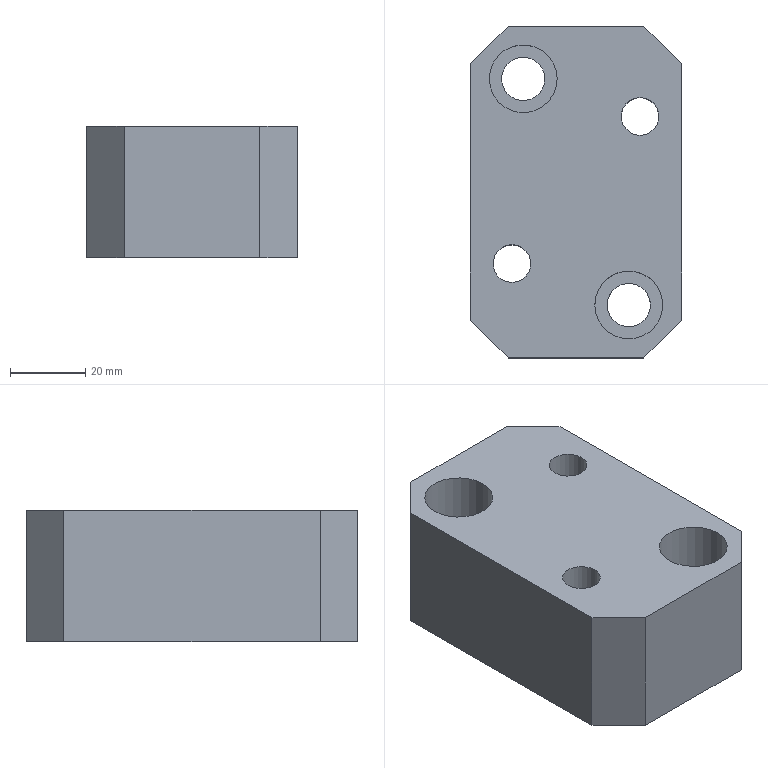Part | NX | features 23 2 | 1 solid | 18 faces | box 56 x 88 x 35 mm | volume 148795 mm3 | plane 12 | cylinder 6 | commonest cylinder face diameters 10.001 x2 11.5 x2 18 x2
STEP:
#1=CARTESIAN_POINT('',(204.592,-285.942,-3.5));
#2=VERTEX_POINT('',#1);
#3=CARTESIAN_POINT('',(209.593,-285.942,-3.5));
#4=DIRECTION('',(0.,0.,-1.));
#5=DIRECTION('',(-1.,0.,0.));
#6=AXIS2_PLACEMENT_3D('',#3,#4,#5);
#7=CIRCLE('',#6,5.);
#8=EDGE_CURVE('',#2,#2,#7,.T.);
#9=ORIENTED_EDGE('',*,*,#8,.T.);
#10=EDGE_LOOP('',(#9));
#11=FACE_BOUND('',#10,.T.);
#12=CARTESIAN_POINT('',(249.593,-296.942,-3.5));
#13=VERTEX_POINT('',#12);
#14=CARTESIAN_POINT('',(240.593,-296.942,-3.5));
#15=DIRECTION('',(0.,0.,1.));
#16=DIRECTION('',(1.,0.,0.));
#17=AXIS2_PLACEMENT_3D('',#14,#15,#16);
#18=CIRCLE('',#17,9.);
#19=EDGE_CURVE('',#13,#13,#18,.T.);
#20=ORIENTED_EDGE('',*,*,#19,.F.);
#21=EDGE_LOOP('',(#20));
#22=FACE_BOUND('',#21,.T.);
#23=CARTESIAN_POINT('',(198.593,-232.942,-3.5));
#24=VERTEX_POINT('',#23);
#25=CARTESIAN_POINT('',(198.593,-300.942,-3.5));
#26=VERTEX_POINT('',#25);
#27=CARTESIAN_POINT('',(198.593,-266.94,-3.5));
#28=DIRECTION('',(0.,-1.,0.));
#29=VECTOR('',#28,1000.);
#30=LINE('',#27,#29);
#31=EDGE_CURVE('',#24,#26,#30,.T.);
#32=ORIENTED_EDGE('',*,*,#31,.T.);
#33=CARTESIAN_POINT('',(208.593,-310.942,-3.5));
#34=VERTEX_POINT('',#33);
#35=CARTESIAN_POINT('',(-31.301,-71.048,-3.5));
#36=DIRECTION('',(0.7071,-0.7071,0.));
#37=VECTOR('',#36,1000.);
#38=LINE('',#35,#37);
#39=EDGE_CURVE('',#26,#34,#38,.T.);
#40=ORIENTED_EDGE('',*,*,#39,.T.);
#41=CARTESIAN_POINT('',(244.593,-310.942,-3.5));
#42=VERTEX_POINT('',#41);
#43=CARTESIAN_POINT('',(226.538,-310.942,-3.5));
#44=DIRECTION('',(1.,0.,0.));
#45=VECTOR('',#44,1000.);
#46=LINE('',#43,#45);
#47=EDGE_CURVE('',#34,#42,#46,.T.);
#48=ORIENTED_EDGE('',*,*,#47,.T.);
#49=CARTESIAN_POINT('',(254.593,-300.942,-3.5));
#50=VERTEX_POINT('',#49);
#51=CARTESIAN_POINT('',(266.966,-288.569,-3.5));
#52=DIRECTION('',(0.7071,0.7071,0.));
#53=VECTOR('',#52,1000.);
#54=LINE('',#51,#53);
#55=EDGE_CURVE('',#42,#50,#54,.T.);
#56=ORIENTED_EDGE('',*,*,#55,.T.);
#57=CARTESIAN_POINT('',(254.593,-232.942,-3.5));
#58=VERTEX_POINT('',#57);
#59=CARTESIAN_POINT('',(254.593,-266.94,-3.5));
#60=DIRECTION('',(0.,1.,0.));
#61=VECTOR('',#60,1000.);
#62=LINE('',#59,#61);
#63=EDGE_CURVE('',#50,#58,#62,.T.);
#64=ORIENTED_EDGE('',*,*,#63,.T.);
#65=CARTESIAN_POINT('',(244.593,-222.942,-3.5));
#66=VERTEX_POINT('',#65);
#67=CARTESIAN_POINT('',(30.699,-9.048,-3.5));
#68=DIRECTION('',(-0.7071,0.7071,0.));
#69=VECTOR('',#68,1000.);
#70=LINE('',#67,#69);
#71=EDGE_CURVE('',#58,#66,#70,.T.);
#72=ORIENTED_EDGE('',*,*,#71,.T.);
#73=CARTESIAN_POINT('',(208.593,-222.942,-3.5));
#74=VERTEX_POINT('',#73);
#75=CARTESIAN_POINT('',(226.538,-222.942,-3.5));
#76=DIRECTION('',(-1.,0.,0.));
#77=VECTOR('',#76,1000.);
#78=LINE('',#75,#77);
#79=EDGE_CURVE('',#66,#74,#78,.T.);
#80=ORIENTED_EDGE('',*,*,#79,.T.);
#81=CARTESIAN_POINT('',(204.966,-226.569,-3.5));
#82=DIRECTION('',(-0.7071,-0.7071,0.));
#83=VECTOR('',#82,1000.);
#84=LINE('',#81,#83);
#85=EDGE_CURVE('',#74,#24,#84,.T.);
#86=ORIENTED_EDGE('',*,*,#85,.T.);
#87=EDGE_LOOP('',(#32,#40,#48,#56,#64,#72,#80,#86));
#88=FACE_BOUND('',#87,.T.);
#89=CARTESIAN_POINT('',(238.592,-246.942,-3.5));
#90=VERTEX_POINT('',#89);
#91=CARTESIAN_POINT('',(243.593,-246.942,-3.5));
#92=DIRECTION('',(0.,0.,-1.));
#93=DIRECTION('',(-1.,0.,0.));
#94=AXIS2_PLACEMENT_3D('',#91,#92,#93);
#95=CIRCLE('',#94,5.);
#96=EDGE_CURVE('',#90,#90,#95,.T.);
#97=ORIENTED_EDGE('',*,*,#96,.T.);
#98=EDGE_LOOP('',(#97));
#99=FACE_BOUND('',#98,.T.);
#100=CARTESIAN_POINT('',(221.593,-236.942,-3.5));
#101=VERTEX_POINT('',#100);
#102=CARTESIAN_POINT('',(212.593,-236.942,-3.5));
#103=DIRECTION('',(0.,0.,1.));
#104=DIRECTION('',(1.,0.,0.));
#105=AXIS2_PLACEMENT_3D('',#102,#103,#104);
#106=CIRCLE('',#105,9.);
#107=EDGE_CURVE('',#101,#101,#106,.T.);
#108=ORIENTED_EDGE('',*,*,#107,.F.);
#109=EDGE_LOOP('',(#108));
#110=FACE_BOUND('',#109,.T.);
#111=CARTESIAN_POINT('',(9.072,-30.675,-3.5));
#112=DIRECTION('',(0.,0.,-1.));
#113=DIRECTION('',(-1.,0.,0.));
#114=AXIS2_PLACEMENT_3D('',#111,#112,#113);
#115=PLANE('',#114);
#116=ADVANCED_FACE('',(#11,#22,#88,#99,#110),#115,.F.);
#117=ORIENTED_EDGE('',*,*,#79,.F.);
#118=CARTESIAN_POINT('',(244.593,-222.942,-38.5));
#119=VERTEX_POINT('',#118);
#120=CARTESIAN_POINT('',(244.593,-222.942,-5.3));
#121=DIRECTION('',(0.,0.,-1.));
#122=VECTOR('',#121,1000.);
#123=LINE('',#120,#122);
#124=EDGE_CURVE('',#66,#119,#123,.T.);
#125=ORIENTED_EDGE('',*,*,#124,.T.);
#126=CARTESIAN_POINT('',(208.593,-222.942,-38.5));
#127=VERTEX_POINT('',#126);
#128=CARTESIAN_POINT('',(226.538,-222.942,-38.5));
#129=DIRECTION('',(1.,0.,0.));
#130=VECTOR('',#129,1000.);
#131=LINE('',#128,#130);
#132=EDGE_CURVE('',#127,#119,#131,.T.);
#133=ORIENTED_EDGE('',*,*,#132,.F.);
#134=CARTESIAN_POINT('',(208.593,-222.942,-5.3));
#135=DIRECTION('',(0.,0.,1.));
#136=VECTOR('',#135,1000.);
#137=LINE('',#134,#136);
#138=EDGE_CURVE('',#127,#74,#137,.T.);
#139=ORIENTED_EDGE('',*,*,#138,.T.);
#140=EDGE_LOOP('',(#117,#125,#133,#139));
#141=FACE_BOUND('',#140,.T.);
#142=CARTESIAN_POINT('',(226.538,-222.942,-5.3));
#143=DIRECTION('',(0.,1.,0.));
#144=DIRECTION('',(0.,0.,1.));
#145=AXIS2_PLACEMENT_3D('',#142,#143,#144);
#146=PLANE('',#145);
#147=ADVANCED_FACE('',(#141),#146,.T.);
#148=CARTESIAN_POINT('',(198.593,-300.942,-38.5));
#149=VERTEX_POINT('',#148);
#150=CARTESIAN_POINT('',(198.593,-232.942,-38.5));
#151=VERTEX_POINT('',#150);
#152=CARTESIAN_POINT('',(198.593,-266.94,-38.5));
#153=DIRECTION('',(0.,1.,0.));
#154=VECTOR('',#153,1000.);
#155=LINE('',#152,#154);
#156=EDGE_CURVE('',#149,#151,#155,.T.);
#157=ORIENTED_EDGE('',*,*,#156,.F.);
#158=CARTESIAN_POINT('',(198.593,-300.942,-5.3));
#159=DIRECTION('',(0.,0.,1.));
#160=VECTOR('',#159,1000.);
#161=LINE('',#158,#160);
#162=EDGE_CURVE('',#149,#26,#161,.T.);
#163=ORIENTED_EDGE('',*,*,#162,.T.);
#164=ORIENTED_EDGE('',*,*,#31,.F.);
#165=CARTESIAN_POINT('',(198.593,-232.942,-5.3));
#166=DIRECTION('',(0.,0.,-1.));
#167=VECTOR('',#166,1000.);
#168=LINE('',#165,#167);
#169=EDGE_CURVE('',#24,#151,#168,.T.);
#170=ORIENTED_EDGE('',*,*,#169,.T.);
#171=EDGE_LOOP('',(#157,#163,#164,#170));
#172=FACE_BOUND('',#171,.T.);
#173=CARTESIAN_POINT('',(198.593,-266.94,-5.3));
#174=DIRECTION('',(-1.,0.,0.));
#175=DIRECTION('',(0.,0.,-1.));
#176=AXIS2_PLACEMENT_3D('',#173,#174,#175);
#177=PLANE('',#176);
#178=ADVANCED_FACE('',(#172),#177,.T.);
#179=ORIENTED_EDGE('',*,*,#47,.F.);
#180=CARTESIAN_POINT('',(208.593,-310.942,-38.5));
#181=VERTEX_POINT('',#180);
#182=CARTESIAN_POINT('',(208.593,-310.942,-5.3));
#183=DIRECTION('',(0.,0.,-1.));
#184=VECTOR('',#183,1000.);
#185=LINE('',#182,#184);
#186=EDGE_CURVE('',#34,#181,#185,.T.);
#187=ORIENTED_EDGE('',*,*,#186,.T.);
#188=CARTESIAN_POINT('',(244.593,-310.942,-38.5));
#189=VERTEX_POINT('',#188);
#190=CARTESIAN_POINT('',(226.538,-310.942,-38.5));
#191=DIRECTION('',(-1.,0.,0.));
#192=VECTOR('',#191,1000.);
#193=LINE('',#190,#192);
#194=EDGE_CURVE('',#189,#181,#193,.T.);
#195=ORIENTED_EDGE('',*,*,#194,.F.);
#196=CARTESIAN_POINT('',(244.593,-310.942,-5.3));
#197=DIRECTION('',(0.,0.,1.));
#198=VECTOR('',#197,1000.);
#199=LINE('',#196,#198);
#200=EDGE_CURVE('',#189,#42,#199,.T.);
#201=ORIENTED_EDGE('',*,*,#200,.T.);
#202=EDGE_LOOP('',(#179,#187,#195,#201));
#203=FACE_BOUND('',#202,.T.);
#204=CARTESIAN_POINT('',(226.538,-310.942,-5.3));
#205=DIRECTION('',(0.,-1.,0.));
#206=DIRECTION('',(0.,0.,-1.));
#207=AXIS2_PLACEMENT_3D('',#204,#205,#206);
#208=PLANE('',#207);
#209=ADVANCED_FACE('',(#203),#208,.T.);
#210=CARTESIAN_POINT('',(204.592,-285.942,-38.5));
#211=VERTEX_POINT('',#210);
#212=CARTESIAN_POINT('',(209.593,-285.942,-38.5));
#213=DIRECTION('',(0.,0.,1.));
#214=DIRECTION('',(-1.,0.,0.));
#215=AXIS2_PLACEMENT_3D('',#212,#213,#214);
#216=CIRCLE('',#215,5.);
#217=EDGE_CURVE('',#211,#211,#216,.T.);
#218=ORIENTED_EDGE('',*,*,#217,.T.);
#219=EDGE_LOOP('',(#218));
#220=FACE_BOUND('',#219,.T.);
#221=CARTESIAN_POINT('',(206.843,-236.942,-38.5));
#222=VERTEX_POINT('',#221);
#223=CARTESIAN_POINT('',(212.593,-236.942,-38.5));
#224=DIRECTION('',(0.,0.,1.));
#225=DIRECTION('',(-1.,0.,0.));
#226=AXIS2_PLACEMENT_3D('',#223,#224,#225);
#227=CIRCLE('',#226,5.75);
#228=EDGE_CURVE('',#222,#222,#227,.T.);
#229=ORIENTED_EDGE('',*,*,#228,.T.);
#230=EDGE_LOOP('',(#229));
#231=FACE_BOUND('',#230,.T.);
#232=CARTESIAN_POINT('',(238.592,-246.942,-38.5));
#233=VERTEX_POINT('',#232);
#234=CARTESIAN_POINT('',(243.593,-246.942,-38.5));
#235=DIRECTION('',(0.,0.,1.));
#236=DIRECTION('',(-1.,0.,0.));
#237=AXIS2_PLACEMENT_3D('',#234,#235,#236);
#238=CIRCLE('',#237,5.);
#239=EDGE_CURVE('',#233,#233,#238,.T.);
#240=ORIENTED_EDGE('',*,*,#239,.T.);
#241=EDGE_LOOP('',(#240));
#242=FACE_BOUND('',#241,.T.);
#243=CARTESIAN_POINT('',(234.843,-296.942,-38.5));
#244=VERTEX_POINT('',#243);
#245=CARTESIAN_POINT('',(240.593,-296.942,-38.5));
#246=DIRECTION('',(0.,0.,1.));
#247=DIRECTION('',(-1.,0.,0.));
#248=AXIS2_PLACEMENT_3D('',#245,#246,#247);
#249=CIRCLE('',#248,5.75);
#250=EDGE_CURVE('',#244,#244,#249,.T.);
#251=ORIENTED_EDGE('',*,*,#250,.T.);
#252=EDGE_LOOP('',(#251));
#253=FACE_BOUND('',#252,.T.);
#254=ORIENTED_EDGE('',*,*,#194,.T.);
#255=CARTESIAN_POINT('',(269.242,-371.591,-38.5));
#256=DIRECTION('',(-0.7071,0.7071,0.));
#257=VECTOR('',#256,1000.);
#258=LINE('',#255,#257);
#259=EDGE_CURVE('',#181,#149,#258,.T.);
#260=ORIENTED_EDGE('',*,*,#259,.T.);
#261=ORIENTED_EDGE('',*,*,#156,.T.);
#262=CARTESIAN_POINT('',(143.46,-288.075,-38.5));
#263=DIRECTION('',(0.7071,0.7071,0.));
#264=VECTOR('',#263,1000.);
#265=LINE('',#262,#264);
#266=EDGE_CURVE('',#151,#127,#265,.T.);
#267=ORIENTED_EDGE('',*,*,#266,.T.);
#268=ORIENTED_EDGE('',*,*,#132,.T.);
#269=CARTESIAN_POINT('',(254.593,-232.942,-38.5));
#270=VERTEX_POINT('',#269);
#271=CARTESIAN_POINT('',(331.242,-309.591,-38.5));
#272=DIRECTION('',(0.7071,-0.7071,0.));
#273=VECTOR('',#272,1000.);
#274=LINE('',#271,#273);
#275=EDGE_CURVE('',#119,#270,#274,.T.);
#276=ORIENTED_EDGE('',*,*,#275,.T.);
#277=CARTESIAN_POINT('',(254.593,-300.942,-38.5));
#278=VERTEX_POINT('',#277);
#279=CARTESIAN_POINT('',(254.593,-266.94,-38.5));
#280=DIRECTION('',(0.,-1.,0.));
#281=VECTOR('',#280,1000.);
#282=LINE('',#279,#281);
#283=EDGE_CURVE('',#270,#278,#282,.T.);
#284=ORIENTED_EDGE('',*,*,#283,.T.);
#285=CARTESIAN_POINT('',(205.46,-350.075,-38.5));
#286=DIRECTION('',(-0.7071,-0.7071,0.));
#287=VECTOR('',#286,1000.);
#288=LINE('',#285,#287);
#289=EDGE_CURVE('',#278,#189,#288,.T.);
#290=ORIENTED_EDGE('',*,*,#289,.T.);
#291=EDGE_LOOP('',(#254,#260,#261,#267,#268,#276,#284,#290));
#292=FACE_BOUND('',#291,.T.);
#293=CARTESIAN_POINT('',(248.109,-392.723,-38.5));
#294=DIRECTION('',(0.,0.,-1.));
#295=DIRECTION('',(-1.,0.,0.));
#296=AXIS2_PLACEMENT_3D('',#293,#294,#295);
#297=PLANE('',#296);
#298=ADVANCED_FACE('',(#220,#231,#242,#253,#292),#297,.T.);
#299=ORIENTED_EDGE('',*,*,#63,.F.);
#300=CARTESIAN_POINT('',(254.593,-300.942,-5.3));
#301=DIRECTION('',(0.,0.,-1.));
#302=VECTOR('',#301,1000.);
#303=LINE('',#300,#302);
#304=EDGE_CURVE('',#50,#278,#303,.T.);
#305=ORIENTED_EDGE('',*,*,#304,.T.);
#306=ORIENTED_EDGE('',*,*,#283,.F.);
#307=CARTESIAN_POINT('',(254.593,-232.942,-5.3));
#308=DIRECTION('',(0.,0.,1.));
#309=VECTOR('',#308,1000.);
#310=LINE('',#307,#309);
#311=EDGE_CURVE('',#270,#58,#310,.T.);
#312=ORIENTED_EDGE('',*,*,#311,.T.);
#313=EDGE_LOOP('',(#299,#305,#306,#312));
#314=FACE_BOUND('',#313,.T.);
#315=CARTESIAN_POINT('',(254.593,-266.94,-5.3));
#316=DIRECTION('',(1.,0.,0.));
#317=DIRECTION('',(0.,0.,1.));
#318=AXIS2_PLACEMENT_3D('',#315,#316,#317);
#319=PLANE('',#318);
#320=ADVANCED_FACE('',(#314),#319,.T.);
#321=ORIENTED_EDGE('',*,*,#250,.F.);
#322=EDGE_LOOP('',(#321));
#323=FACE_BOUND('',#322,.T.);
#324=CARTESIAN_POINT('',(234.843,-296.942,-16.5));
#325=VERTEX_POINT('',#324);
#326=CARTESIAN_POINT('',(240.593,-296.942,-16.5));
#327=DIRECTION('',(0.,0.,1.));
#328=DIRECTION('',(-1.,0.,0.));
#329=AXIS2_PLACEMENT_3D('',#326,#327,#328);
#330=CIRCLE('',#329,5.75);
#331=EDGE_CURVE('',#325,#325,#330,.T.);
#332=ORIENTED_EDGE('',*,*,#331,.T.);
#333=EDGE_LOOP('',(#332));
#334=FACE_BOUND('',#333,.T.);
#335=CARTESIAN_POINT('',(240.593,-296.942,-1.5));
#336=DIRECTION('',(0.,0.,-1.));
#337=DIRECTION('',(-1.,0.,0.));
#338=AXIS2_PLACEMENT_3D('',#335,#336,#337);
#339=CYLINDRICAL_SURFACE('',#338,5.75);
#340=ADVANCED_FACE('',(#323,#334),#339,.F.);
#341=ORIENTED_EDGE('',*,*,#331,.F.);
#342=EDGE_LOOP('',(#341));
#343=FACE_BOUND('',#342,.T.);
#344=CARTESIAN_POINT('',(249.593,-296.942,-16.5));
#345=VERTEX_POINT('',#344);
#346=CARTESIAN_POINT('',(240.593,-296.942,-16.5));
#347=DIRECTION('',(0.,0.,1.));
#348=DIRECTION('',(1.,0.,0.));
#349=AXIS2_PLACEMENT_3D('',#346,#347,#348);
#350=CIRCLE('',#349,9.);
#351=EDGE_CURVE('',#345,#345,#350,.T.);
#352=ORIENTED_EDGE('',*,*,#351,.T.);
#353=EDGE_LOOP('',(#352));
#354=FACE_BOUND('',#353,.T.);
#355=CARTESIAN_POINT('',(240.593,-296.942,-16.5));
#356=DIRECTION('',(0.,0.,-1.));
#357=DIRECTION('',(1.,0.,0.));
#358=AXIS2_PLACEMENT_3D('',#355,#356,#357);
#359=PLANE('',#358);
#360=ADVANCED_FACE('',(#343,#354),#359,.F.);
#361=ORIENTED_EDGE('',*,*,#351,.F.);
#362=EDGE_LOOP('',(#361));
#363=FACE_BOUND('',#362,.T.);
#364=ORIENTED_EDGE('',*,*,#19,.T.);
#365=EDGE_LOOP('',(#364));
#366=FACE_BOUND('',#365,.T.);
#367=CARTESIAN_POINT('',(240.593,-296.942,-3.5));
#368=DIRECTION('',(0.,0.,-1.));
#369=DIRECTION('',(-1.,0.,0.));
#370=AXIS2_PLACEMENT_3D('',#367,#368,#369);
#371=CYLINDRICAL_SURFACE('',#370,9.);
#372=ADVANCED_FACE('',(#363,#366),#371,.F.);
#373=ORIENTED_EDGE('',*,*,#96,.F.);
#374=EDGE_LOOP('',(#373));
#375=FACE_BOUND('',#374,.T.);
#376=ORIENTED_EDGE('',*,*,#239,.F.);
#377=EDGE_LOOP('',(#376));
#378=FACE_BOUND('',#377,.T.);
#379=CARTESIAN_POINT('',(243.593,-246.942,-1.5));
#380=DIRECTION('',(0.,0.,-1.));
#381=DIRECTION('',(-1.,0.,0.));
#382=AXIS2_PLACEMENT_3D('',#379,#380,#381);
#383=CYLINDRICAL_SURFACE('',#382,5.);
#384=ADVANCED_FACE('',(#375,#378),#383,.F.);
#385=ORIENTED_EDGE('',*,*,#228,.F.);
#386=EDGE_LOOP('',(#385));
#387=FACE_BOUND('',#386,.T.);
#388=CARTESIAN_POINT('',(206.843,-236.942,-16.5));
#389=VERTEX_POINT('',#388);
#390=CARTESIAN_POINT('',(212.593,-236.942,-16.5));
#391=DIRECTION('',(0.,0.,1.));
#392=DIRECTION('',(-1.,0.,0.));
#393=AXIS2_PLACEMENT_3D('',#390,#391,#392);
#394=CIRCLE('',#393,5.75);
#395=EDGE_CURVE('',#389,#389,#394,.T.);
#396=ORIENTED_EDGE('',*,*,#395,.T.);
#397=EDGE_LOOP('',(#396));
#398=FACE_BOUND('',#397,.T.);
#399=CARTESIAN_POINT('',(212.593,-236.942,-1.5));
#400=DIRECTION('',(0.,0.,-1.));
#401=DIRECTION('',(-1.,0.,0.));
#402=AXIS2_PLACEMENT_3D('',#399,#400,#401);
#403=CYLINDRICAL_SURFACE('',#402,5.75);
#404=ADVANCED_FACE('',(#387,#398),#403,.F.);
#405=ORIENTED_EDGE('',*,*,#395,.F.);
#406=EDGE_LOOP('',(#405));
#407=FACE_BOUND('',#406,.T.);
#408=CARTESIAN_POINT('',(221.593,-236.942,-16.5));
#409=VERTEX_POINT('',#408);
#410=CARTESIAN_POINT('',(212.593,-236.942,-16.5));
#411=DIRECTION('',(0.,0.,1.));
#412=DIRECTION('',(1.,0.,0.));
#413=AXIS2_PLACEMENT_3D('',#410,#411,#412);
#414=CIRCLE('',#413,9.);
#415=EDGE_CURVE('',#409,#409,#414,.T.);
#416=ORIENTED_EDGE('',*,*,#415,.T.);
#417=EDGE_LOOP('',(#416));
#418=FACE_BOUND('',#417,.T.);
#419=CARTESIAN_POINT('',(212.593,-236.942,-16.5));
#420=DIRECTION('',(0.,0.,-1.));
#421=DIRECTION('',(1.,0.,0.));
#422=AXIS2_PLACEMENT_3D('',#419,#420,#421);
#423=PLANE('',#422);
#424=ADVANCED_FACE('',(#407,#418),#423,.F.);
#425=ORIENTED_EDGE('',*,*,#415,.F.);
#426=EDGE_LOOP('',(#425));
#427=FACE_BOUND('',#426,.T.);
#428=ORIENTED_EDGE('',*,*,#107,.T.);
#429=EDGE_LOOP('',(#428));
#430=FACE_BOUND('',#429,.T.);
#431=CARTESIAN_POINT('',(212.593,-236.942,-3.5));
#432=DIRECTION('',(0.,0.,-1.));
#433=DIRECTION('',(-1.,0.,0.));
#434=AXIS2_PLACEMENT_3D('',#431,#432,#433);
#435=CYLINDRICAL_SURFACE('',#434,9.);
#436=ADVANCED_FACE('',(#427,#430),#435,.F.);
#437=ORIENTED_EDGE('',*,*,#8,.F.);
#438=EDGE_LOOP('',(#437));
#439=FACE_BOUND('',#438,.T.);
#440=ORIENTED_EDGE('',*,*,#217,.F.);
#441=EDGE_LOOP('',(#440));
#442=FACE_BOUND('',#441,.T.);
#443=CARTESIAN_POINT('',(209.593,-285.942,-1.5));
#444=DIRECTION('',(0.,0.,-1.));
#445=DIRECTION('',(-1.,0.,0.));
#446=AXIS2_PLACEMENT_3D('',#443,#444,#445);
#447=CYLINDRICAL_SURFACE('',#446,5.);
#448=ADVANCED_FACE('',(#439,#442),#447,.F.);
#449=ORIENTED_EDGE('',*,*,#259,.F.);
#450=ORIENTED_EDGE('',*,*,#186,.F.);
#451=ORIENTED_EDGE('',*,*,#39,.F.);
#452=ORIENTED_EDGE('',*,*,#162,.F.);
#453=EDGE_LOOP('',(#449,#450,#451,#452));
#454=FACE_BOUND('',#453,.T.);
#455=CARTESIAN_POINT('',(198.593,-300.942,-5.3));
#456=DIRECTION('',(0.7071,0.7071,0.));
#457=DIRECTION('',(0.,0.,-1.));
#458=AXIS2_PLACEMENT_3D('',#455,#456,#457);
#459=PLANE('',#458);
#460=ADVANCED_FACE('',(#454),#459,.F.);
#461=ORIENTED_EDGE('',*,*,#289,.F.);
#462=ORIENTED_EDGE('',*,*,#304,.F.);
#463=ORIENTED_EDGE('',*,*,#55,.F.);
#464=ORIENTED_EDGE('',*,*,#200,.F.);
#465=EDGE_LOOP('',(#461,#462,#463,#464));
#466=FACE_BOUND('',#465,.T.);
#467=CARTESIAN_POINT('',(244.593,-310.942,-5.3));
#468=DIRECTION('',(-0.7071,0.7071,0.));
#469=DIRECTION('',(0.,0.,-1.));
#470=AXIS2_PLACEMENT_3D('',#467,#468,#469);
#471=PLANE('',#470);
#472=ADVANCED_FACE('',(#466),#471,.F.);
#473=ORIENTED_EDGE('',*,*,#275,.F.);
#474=ORIENTED_EDGE('',*,*,#124,.F.);
#475=ORIENTED_EDGE('',*,*,#71,.F.);
#476=ORIENTED_EDGE('',*,*,#311,.F.);
#477=EDGE_LOOP('',(#473,#474,#475,#476));
#478=FACE_BOUND('',#477,.T.);
#479=CARTESIAN_POINT('',(254.593,-232.942,-5.3));
#480=DIRECTION('',(-0.7071,-0.7071,0.));
#481=DIRECTION('',(0.,0.,-1.));
#482=AXIS2_PLACEMENT_3D('',#479,#480,#481);
#483=PLANE('',#482);
#484=ADVANCED_FACE('',(#478),#483,.F.);
#485=ORIENTED_EDGE('',*,*,#266,.F.);
#486=ORIENTED_EDGE('',*,*,#169,.F.);
#487=ORIENTED_EDGE('',*,*,#85,.F.);
#488=ORIENTED_EDGE('',*,*,#138,.F.);
#489=EDGE_LOOP('',(#485,#486,#487,#488));
#490=FACE_BOUND('',#489,.T.);
#491=CARTESIAN_POINT('',(208.593,-222.942,-5.3));
#492=DIRECTION('',(0.7071,-0.7071,0.));
#493=DIRECTION('',(0.,0.,-1.));
#494=AXIS2_PLACEMENT_3D('',#491,#492,#493);
#495=PLANE('',#494);
#496=ADVANCED_FACE('',(#490),#495,.F.);
#497=CLOSED_SHELL('',(#116,#147,#178,#209,#298,#320,#340,#360,#372,#384,#404,#424,#436,#448,#460,#472,#484,#496));
#498=MANIFOLD_SOLID_BREP('',#497);
#499=(LENGTH_UNIT()NAMED_UNIT(*)SI_UNIT(.MILLI.,.METRE.));
#500=UNCERTAINTY_MEASURE_WITH_UNIT(LENGTH_MEASURE(0.00001),#499,'','');
#501=(NAMED_UNIT(*)PLANE_ANGLE_UNIT()SI_UNIT($,.RADIAN.));
#502=(NAMED_UNIT(*)SI_UNIT($,.STERADIAN.)SOLID_ANGLE_UNIT());
#503=(GEOMETRIC_REPRESENTATION_CONTEXT(3)GLOBAL_UNCERTAINTY_ASSIGNED_CONTEXT((#500))GLOBAL_UNIT_ASSIGNED_CONTEXT((#499,#501,#502))REPRESENTATION_CONTEXT('',''));
#504=ADVANCED_BREP_SHAPE_REPRESENTATION('',(#498),#503);